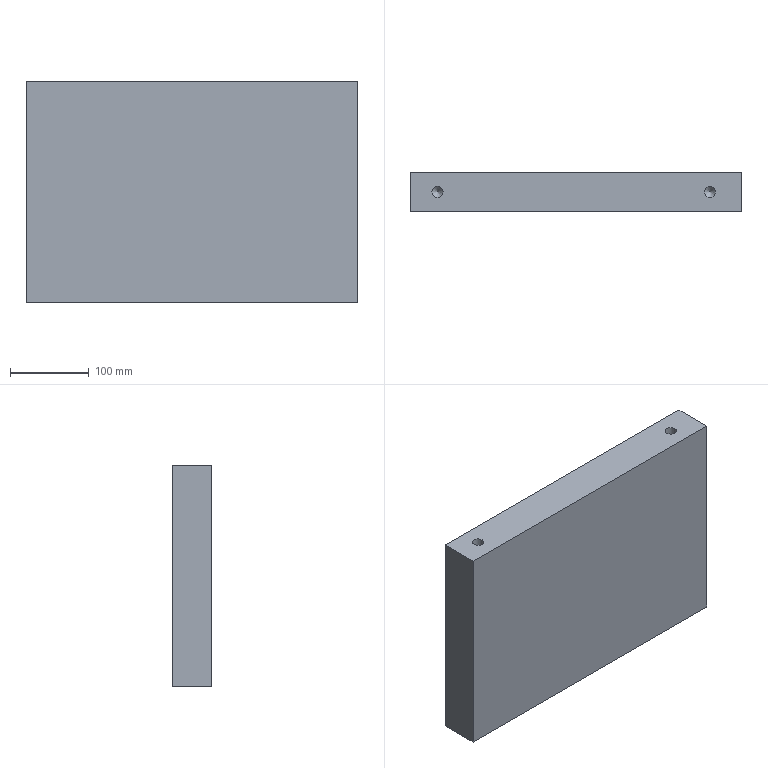Part | NX | features 29 2 | 1 solid | 14 faces | box 418.676 x 50 x 280.5 mm | volume 5847390 mm3 | plane 6 | cylinder 4 | cone 4 | commonest cylinder face diameters 14.1 x4
STEP:
#1=CARTESIAN_POINT('',(519.712,-303.162,-493.5));
#2=VERTEX_POINT('',#1);
#3=CARTESIAN_POINT('',(512.662,-303.162,-493.5));
#4=DIRECTION('',(0.,0.,1.));
#5=DIRECTION('',(1.,0.,0.));
#6=AXIS2_PLACEMENT_3D('',#3,#4,#5);
#7=CIRCLE('',#6,7.05);
#8=EDGE_CURVE('',#2,#2,#7,.T.);
#9=ORIENTED_EDGE('',*,*,#8,.T.);
#10=EDGE_LOOP('',(#9));
#11=FACE_BOUND('',#10,.T.);
#12=CARTESIAN_POINT('',(552.338,-278.162,-493.5));
#13=VERTEX_POINT('',#12);
#14=CARTESIAN_POINT('',(133.662,-278.162,-493.5));
#15=VERTEX_POINT('',#14);
#16=CARTESIAN_POINT('',(-123.162,-278.162,-493.5));
#17=DIRECTION('',(-1.,0.,0.));
#18=VECTOR('',#17,1000.);
#19=LINE('',#16,#18);
#20=EDGE_CURVE('',#13,#15,#19,.T.);
#21=ORIENTED_EDGE('',*,*,#20,.F.);
#22=CARTESIAN_POINT('',(552.338,-328.162,-493.5));
#23=VERTEX_POINT('',#22);
#24=CARTESIAN_POINT('',(552.338,226.838,-493.5));
#25=DIRECTION('',(0.,-1.,0.));
#26=VECTOR('',#25,1000.);
#27=LINE('',#24,#26);
#28=EDGE_CURVE('',#13,#23,#27,.T.);
#29=ORIENTED_EDGE('',*,*,#28,.T.);
#30=CARTESIAN_POINT('',(133.662,-328.162,-493.5));
#31=VERTEX_POINT('',#30);
#32=CARTESIAN_POINT('',(-123.162,-328.162,-493.5));
#33=DIRECTION('',(1.,0.,0.));
#34=VECTOR('',#33,1000.);
#35=LINE('',#32,#34);
#36=EDGE_CURVE('',#31,#23,#35,.T.);
#37=ORIENTED_EDGE('',*,*,#36,.F.);
#38=CARTESIAN_POINT('',(133.662,190.823,-493.5));
#39=DIRECTION('',(0.,-1.,0.));
#40=VECTOR('',#39,1000.);
#41=LINE('',#38,#40);
#42=EDGE_CURVE('',#15,#31,#41,.T.);
#43=ORIENTED_EDGE('',*,*,#42,.F.);
#44=EDGE_LOOP('',(#21,#29,#37,#43));
#45=FACE_BOUND('',#44,.T.);
#46=CARTESIAN_POINT('',(174.712,-303.162,-493.5));
#47=VERTEX_POINT('',#46);
#48=CARTESIAN_POINT('',(167.662,-303.162,-493.5));
#49=DIRECTION('',(0.,0.,1.));
#50=DIRECTION('',(1.,0.,0.));
#51=AXIS2_PLACEMENT_3D('',#48,#49,#50);
#52=CIRCLE('',#51,7.05);
#53=EDGE_CURVE('',#47,#47,#52,.T.);
#54=ORIENTED_EDGE('',*,*,#53,.T.);
#55=EDGE_LOOP('',(#54));
#56=FACE_BOUND('',#55,.T.);
#57=CARTESIAN_POINT('',(69.838,1108.838,-493.5));
#58=DIRECTION('',(0.,0.,-1.));
#59=DIRECTION('',(0.,1.,0.));
#60=AXIS2_PLACEMENT_3D('',#57,#58,#59);
#61=PLANE('',#60);
#62=ADVANCED_FACE('',(#11,#45,#56),#61,.T.);
#63=CARTESIAN_POINT('',(519.712,-303.162,-213.));
#64=VERTEX_POINT('',#63);
#65=CARTESIAN_POINT('',(512.662,-303.162,-213.));
#66=DIRECTION('',(0.,0.,-1.));
#67=DIRECTION('',(1.,0.,0.));
#68=AXIS2_PLACEMENT_3D('',#65,#66,#67);
#69=CIRCLE('',#68,7.05);
#70=EDGE_CURVE('',#64,#64,#69,.T.);
#71=ORIENTED_EDGE('',*,*,#70,.T.);
#72=EDGE_LOOP('',(#71));
#73=FACE_BOUND('',#72,.T.);
#74=CARTESIAN_POINT('',(133.662,-278.162,-213.));
#75=VERTEX_POINT('',#74);
#76=CARTESIAN_POINT('',(552.338,-278.162,-213.));
#77=VERTEX_POINT('',#76);
#78=CARTESIAN_POINT('',(-123.162,-278.162,-213.));
#79=DIRECTION('',(1.,0.,0.));
#80=VECTOR('',#79,1000.);
#81=LINE('',#78,#80);
#82=EDGE_CURVE('',#75,#77,#81,.T.);
#83=ORIENTED_EDGE('',*,*,#82,.F.);
#84=CARTESIAN_POINT('',(133.662,-328.162,-213.));
#85=VERTEX_POINT('',#84);
#86=CARTESIAN_POINT('',(133.662,190.823,-213.));
#87=DIRECTION('',(0.,1.,0.));
#88=VECTOR('',#87,1000.);
#89=LINE('',#86,#88);
#90=EDGE_CURVE('',#85,#75,#89,.T.);
#91=ORIENTED_EDGE('',*,*,#90,.F.);
#92=CARTESIAN_POINT('',(552.338,-328.162,-213.));
#93=VERTEX_POINT('',#92);
#94=CARTESIAN_POINT('',(-123.162,-328.162,-213.));
#95=DIRECTION('',(-1.,0.,0.));
#96=VECTOR('',#95,1000.);
#97=LINE('',#94,#96);
#98=EDGE_CURVE('',#93,#85,#97,.T.);
#99=ORIENTED_EDGE('',*,*,#98,.F.);
#100=CARTESIAN_POINT('',(552.338,226.838,-213.));
#101=DIRECTION('',(0.,1.,0.));
#102=VECTOR('',#101,1000.);
#103=LINE('',#100,#102);
#104=EDGE_CURVE('',#93,#77,#103,.T.);
#105=ORIENTED_EDGE('',*,*,#104,.T.);
#106=EDGE_LOOP('',(#83,#91,#99,#105));
#107=FACE_BOUND('',#106,.T.);
#108=CARTESIAN_POINT('',(174.712,-303.162,-213.));
#109=VERTEX_POINT('',#108);
#110=CARTESIAN_POINT('',(167.662,-303.162,-213.));
#111=DIRECTION('',(0.,0.,-1.));
#112=DIRECTION('',(1.,0.,0.));
#113=AXIS2_PLACEMENT_3D('',#110,#111,#112);
#114=CIRCLE('',#113,7.05);
#115=EDGE_CURVE('',#109,#109,#114,.T.);
#116=ORIENTED_EDGE('',*,*,#115,.T.);
#117=EDGE_LOOP('',(#116));
#118=FACE_BOUND('',#117,.T.);
#119=CARTESIAN_POINT('',(69.838,1108.838,-213.));
#120=DIRECTION('',(0.,0.,1.));
#121=DIRECTION('',(0.,-1.,0.));
#122=AXIS2_PLACEMENT_3D('',#119,#120,#121);
#123=PLANE('',#122);
#124=ADVANCED_FACE('',(#73,#107,#118),#123,.T.);
#125=CARTESIAN_POINT('',(133.662,-278.162,0.));
#126=DIRECTION('',(0.,0.,-1.));
#127=VECTOR('',#126,1000.);
#128=LINE('',#125,#127);
#129=EDGE_CURVE('',#75,#15,#128,.T.);
#130=ORIENTED_EDGE('',*,*,#129,.T.);
#131=ORIENTED_EDGE('',*,*,#42,.T.);
#132=CARTESIAN_POINT('',(133.662,-328.162,-205.5));
#133=DIRECTION('',(0.,0.,-1.));
#134=VECTOR('',#133,1000.);
#135=LINE('',#132,#134);
#136=EDGE_CURVE('',#85,#31,#135,.T.);
#137=ORIENTED_EDGE('',*,*,#136,.F.);
#138=ORIENTED_EDGE('',*,*,#90,.T.);
#139=EDGE_LOOP('',(#130,#131,#137,#138));
#140=FACE_BOUND('',#139,.T.);
#141=CARTESIAN_POINT('',(133.662,190.823,0.));
#142=DIRECTION('',(-1.,0.,0.));
#143=DIRECTION('',(0.,0.,-1.));
#144=AXIS2_PLACEMENT_3D('',#141,#142,#143);
#145=PLANE('',#144);
#146=ADVANCED_FACE('',(#140),#145,.T.);
#147=ORIENTED_EDGE('',*,*,#28,.F.);
#148=CARTESIAN_POINT('',(552.338,-278.162,-205.5));
#149=DIRECTION('',(0.,0.,1.));
#150=VECTOR('',#149,1000.);
#151=LINE('',#148,#150);
#152=EDGE_CURVE('',#13,#77,#151,.T.);
#153=ORIENTED_EDGE('',*,*,#152,.T.);
#154=ORIENTED_EDGE('',*,*,#104,.F.);
#155=CARTESIAN_POINT('',(552.338,-328.162,-113.));
#156=DIRECTION('',(0.,0.,1.));
#157=VECTOR('',#156,1000.);
#158=LINE('',#155,#157);
#159=EDGE_CURVE('',#23,#93,#158,.T.);
#160=ORIENTED_EDGE('',*,*,#159,.F.);
#161=EDGE_LOOP('',(#147,#153,#154,#160));
#162=FACE_BOUND('',#161,.T.);
#163=CARTESIAN_POINT('',(552.338,226.838,-113.));
#164=DIRECTION('',(-1.,0.,0.));
#165=DIRECTION('',(0.,1.,0.));
#166=AXIS2_PLACEMENT_3D('',#163,#164,#165);
#167=PLANE('',#166);
#168=ADVANCED_FACE('',(#162),#167,.F.);
#169=ORIENTED_EDGE('',*,*,#152,.F.);
#170=ORIENTED_EDGE('',*,*,#20,.T.);
#171=ORIENTED_EDGE('',*,*,#129,.F.);
#172=ORIENTED_EDGE('',*,*,#82,.T.);
#173=EDGE_LOOP('',(#169,#170,#171,#172));
#174=FACE_BOUND('',#173,.T.);
#175=CARTESIAN_POINT('',(-123.162,-278.162,-205.5));
#176=DIRECTION('',(0.,1.,0.));
#177=DIRECTION('',(0.,0.,-1.));
#178=AXIS2_PLACEMENT_3D('',#175,#176,#177);
#179=PLANE('',#178);
#180=ADVANCED_FACE('',(#174),#179,.T.);
#181=ORIENTED_EDGE('',*,*,#136,.T.);
#182=ORIENTED_EDGE('',*,*,#36,.T.);
#183=ORIENTED_EDGE('',*,*,#159,.T.);
#184=ORIENTED_EDGE('',*,*,#98,.T.);
#185=EDGE_LOOP('',(#181,#182,#183,#184));
#186=FACE_BOUND('',#185,.T.);
#187=CARTESIAN_POINT('',(-123.162,-328.162,-205.5));
#188=DIRECTION('',(0.,-1.,0.));
#189=DIRECTION('',(0.,0.,1.));
#190=AXIS2_PLACEMENT_3D('',#187,#188,#189);
#191=PLANE('',#190);
#192=ADVANCED_FACE('',(#186),#191,.T.);
#193=CARTESIAN_POINT('',(505.612,-303.162,-249.95));
#194=VERTEX_POINT('',#193);
#195=CARTESIAN_POINT('',(512.662,-303.162,-249.95));
#196=DIRECTION('',(0.,0.,-1.));
#197=DIRECTION('',(-1.,0.,0.));
#198=AXIS2_PLACEMENT_3D('',#195,#196,#197);
#199=CIRCLE('',#198,7.05);
#200=EDGE_CURVE('',#194,#194,#199,.T.);
#201=ORIENTED_EDGE('',*,*,#200,.T.);
#202=EDGE_LOOP('',(#201));
#203=FACE_BOUND('',#202,.T.);
#204=ORIENTED_EDGE('',*,*,#70,.F.);
#205=EDGE_LOOP('',(#204));
#206=FACE_BOUND('',#205,.T.);
#207=CARTESIAN_POINT('',(512.662,-303.162,-213.));
#208=DIRECTION('',(0.,0.,-1.));
#209=DIRECTION('',(-1.,0.,0.));
#210=AXIS2_PLACEMENT_3D('',#207,#208,#209);
#211=CYLINDRICAL_SURFACE('',#210,7.05);
#212=ADVANCED_FACE('',(#203,#206),#211,.F.);
#213=CARTESIAN_POINT('',(512.662,-303.162,-257.));
#214=VERTEX_POINT('',#213);
#215=VERTEX_LOOP('',#214);
#216=FACE_BOUND('',#215,.T.);
#217=ORIENTED_EDGE('',*,*,#200,.F.);
#218=EDGE_LOOP('',(#217));
#219=FACE_BOUND('',#218,.T.);
#220=CARTESIAN_POINT('',(512.662,-303.162,-249.95));
#221=DIRECTION('',(0.,0.,1.));
#222=DIRECTION('',(-1.,0.,0.));
#223=AXIS2_PLACEMENT_3D('',#220,#221,#222);
#224=CONICAL_SURFACE('',#223,7.05,0.7854);
#225=ADVANCED_FACE('',(#216,#219),#224,.F.);
#226=CARTESIAN_POINT('',(160.612,-303.162,-249.95));
#227=VERTEX_POINT('',#226);
#228=CARTESIAN_POINT('',(167.662,-303.162,-249.95));
#229=DIRECTION('',(0.,0.,-1.));
#230=DIRECTION('',(-1.,0.,0.));
#231=AXIS2_PLACEMENT_3D('',#228,#229,#230);
#232=CIRCLE('',#231,7.05);
#233=EDGE_CURVE('',#227,#227,#232,.T.);
#234=ORIENTED_EDGE('',*,*,#233,.T.);
#235=EDGE_LOOP('',(#234));
#236=FACE_BOUND('',#235,.T.);
#237=ORIENTED_EDGE('',*,*,#115,.F.);
#238=EDGE_LOOP('',(#237));
#239=FACE_BOUND('',#238,.T.);
#240=CARTESIAN_POINT('',(167.662,-303.162,-213.));
#241=DIRECTION('',(0.,0.,-1.));
#242=DIRECTION('',(-1.,0.,0.));
#243=AXIS2_PLACEMENT_3D('',#240,#241,#242);
#244=CYLINDRICAL_SURFACE('',#243,7.05);
#245=ADVANCED_FACE('',(#236,#239),#244,.F.);
#246=CARTESIAN_POINT('',(167.662,-303.162,-257.));
#247=VERTEX_POINT('',#246);
#248=VERTEX_LOOP('',#247);
#249=FACE_BOUND('',#248,.T.);
#250=ORIENTED_EDGE('',*,*,#233,.F.);
#251=EDGE_LOOP('',(#250));
#252=FACE_BOUND('',#251,.T.);
#253=CARTESIAN_POINT('',(167.662,-303.162,-249.95));
#254=DIRECTION('',(0.,0.,1.));
#255=DIRECTION('',(-1.,0.,0.));
#256=AXIS2_PLACEMENT_3D('',#253,#254,#255);
#257=CONICAL_SURFACE('',#256,7.05,0.7854);
#258=ADVANCED_FACE('',(#249,#252),#257,.F.);
#259=CARTESIAN_POINT('',(519.712,-303.162,-456.55));
#260=VERTEX_POINT('',#259);
#261=CARTESIAN_POINT('',(512.662,-303.162,-456.55));
#262=DIRECTION('',(0.,0.,1.));
#263=DIRECTION('',(1.,0.,0.));
#264=AXIS2_PLACEMENT_3D('',#261,#262,#263);
#265=CIRCLE('',#264,7.05);
#266=EDGE_CURVE('',#260,#260,#265,.T.);
#267=ORIENTED_EDGE('',*,*,#266,.T.);
#268=EDGE_LOOP('',(#267));
#269=FACE_BOUND('',#268,.T.);
#270=ORIENTED_EDGE('',*,*,#8,.F.);
#271=EDGE_LOOP('',(#270));
#272=FACE_BOUND('',#271,.T.);
#273=CARTESIAN_POINT('',(512.662,-303.162,-493.5));
#274=DIRECTION('',(0.,0.,1.));
#275=DIRECTION('',(-1.,0.,0.));
#276=AXIS2_PLACEMENT_3D('',#273,#274,#275);
#277=CYLINDRICAL_SURFACE('',#276,7.05);
#278=ADVANCED_FACE('',(#269,#272),#277,.F.);
#279=CARTESIAN_POINT('',(512.662,-303.162,-449.5));
#280=VERTEX_POINT('',#279);
#281=VERTEX_LOOP('',#280);
#282=FACE_BOUND('',#281,.T.);
#283=ORIENTED_EDGE('',*,*,#266,.F.);
#284=EDGE_LOOP('',(#283));
#285=FACE_BOUND('',#284,.T.);
#286=CARTESIAN_POINT('',(512.662,-303.162,-456.55));
#287=DIRECTION('',(0.,0.,-1.));
#288=DIRECTION('',(1.,0.,0.));
#289=AXIS2_PLACEMENT_3D('',#286,#287,#288);
#290=CONICAL_SURFACE('',#289,7.05,0.7854);
#291=ADVANCED_FACE('',(#282,#285),#290,.F.);
#292=CARTESIAN_POINT('',(174.712,-303.162,-456.55));
#293=VERTEX_POINT('',#292);
#294=CARTESIAN_POINT('',(167.662,-303.162,-456.55));
#295=DIRECTION('',(0.,0.,1.));
#296=DIRECTION('',(1.,0.,0.));
#297=AXIS2_PLACEMENT_3D('',#294,#295,#296);
#298=CIRCLE('',#297,7.05);
#299=EDGE_CURVE('',#293,#293,#298,.T.);
#300=ORIENTED_EDGE('',*,*,#299,.T.);
#301=EDGE_LOOP('',(#300));
#302=FACE_BOUND('',#301,.T.);
#303=ORIENTED_EDGE('',*,*,#53,.F.);
#304=EDGE_LOOP('',(#303));
#305=FACE_BOUND('',#304,.T.);
#306=CARTESIAN_POINT('',(167.662,-303.162,-493.5));
#307=DIRECTION('',(0.,0.,1.));
#308=DIRECTION('',(-1.,0.,0.));
#309=AXIS2_PLACEMENT_3D('',#306,#307,#308);
#310=CYLINDRICAL_SURFACE('',#309,7.05);
#311=ADVANCED_FACE('',(#302,#305),#310,.F.);
#312=CARTESIAN_POINT('',(167.662,-303.162,-449.5));
#313=VERTEX_POINT('',#312);
#314=VERTEX_LOOP('',#313);
#315=FACE_BOUND('',#314,.T.);
#316=ORIENTED_EDGE('',*,*,#299,.F.);
#317=EDGE_LOOP('',(#316));
#318=FACE_BOUND('',#317,.T.);
#319=CARTESIAN_POINT('',(167.662,-303.162,-456.55));
#320=DIRECTION('',(0.,0.,-1.));
#321=DIRECTION('',(1.,0.,0.));
#322=AXIS2_PLACEMENT_3D('',#319,#320,#321);
#323=CONICAL_SURFACE('',#322,7.05,0.7854);
#324=ADVANCED_FACE('',(#315,#318),#323,.F.);
#325=CLOSED_SHELL('',(#62,#124,#146,#168,#180,#192,#212,#225,#245,#258,#278,#291,#311,#324));
#326=MANIFOLD_SOLID_BREP('',#325);
#327=(LENGTH_UNIT()NAMED_UNIT(*)SI_UNIT(.MILLI.,.METRE.));
#328=UNCERTAINTY_MEASURE_WITH_UNIT(LENGTH_MEASURE(0.00001),#327,'','');
#329=(NAMED_UNIT(*)PLANE_ANGLE_UNIT()SI_UNIT($,.RADIAN.));
#330=(NAMED_UNIT(*)SI_UNIT($,.STERADIAN.)SOLID_ANGLE_UNIT());
#331=(GEOMETRIC_REPRESENTATION_CONTEXT(3)GLOBAL_UNCERTAINTY_ASSIGNED_CONTEXT((#328))GLOBAL_UNIT_ASSIGNED_CONTEXT((#327,#329,#330))REPRESENTATION_CONTEXT('',''));
#332=ADVANCED_BREP_SHAPE_REPRESENTATION('',(#326),#331);